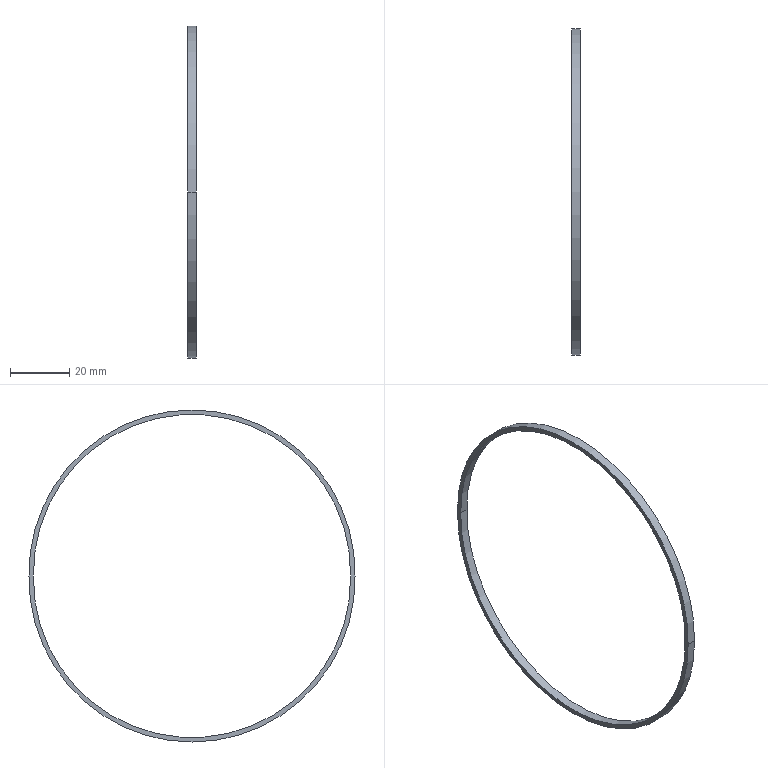Part | STEP file | 1-56.28 | 1 solid | 6 faces | box 3 x 110 x 112 mm | volume 1552 mm3 | cylinder 4 | plane 2 | commonest cylinder face diameters 107 x2 110 x2
STEP:
#1=CARTESIAN_POINT('',(0.,0.,0.));
#2=DIRECTION('',(0.,0.,1.));
#3=DIRECTION('',(1.,0.,0.));
#4=AXIS2_PLACEMENT_3D('',#1,#2,#3);
#5=CARTESIAN_POINT('',(0.,54.991,-1.));
#6=VERTEX_POINT('',#5);
#7=CARTESIAN_POINT('',(0.,-54.991,-1.));
#8=VERTEX_POINT('',#7);
#9=CARTESIAN_POINT('',(0.,0.,0.));
#10=DIRECTION('',(1.,0.,0.));
#11=DIRECTION('',(0.,0.9998,-0.01818));
#12=AXIS2_PLACEMENT_3D('',#9,#10,#11);
#13=CIRCLE('',#12,55.);
#14=CARTESIAN_POINT('',(0.,0.,-0.9907));
#15=DIRECTION('',(1.,0.,0.));
#16=DIRECTION('',(0.,1.,0.));
#17=AXIS2_PLACEMENT_3D('',#14,#15,#16);
#18=PLANE('',#17);
#19=CARTESIAN_POINT('',(0.,0.9907));
#20=DIRECTION('',(0.9998,-0.01818));
#21=AXIS2_PLACEMENT_2D('',#19,#20);
#22=CIRCLE('',#21,55.);
#23=(GEOMETRIC_REPRESENTATION_CONTEXT(2)PARAMETRIC_REPRESENTATION_CONTEXT()REPRESENTATION_CONTEXT('',''));
#24=DEFINITIONAL_REPRESENTATION('',(#22),#23);
#25=PCURVE('',#18,#24);
#26=CARTESIAN_POINT('',(0.,0.,0.));
#27=DIRECTION('',(1.,0.,0.));
#28=DIRECTION('',(0.,0.9998,-0.01818));
#29=AXIS2_PLACEMENT_3D('',#26,#27,#28);
#30=CYLINDRICAL_SURFACE('',#29,55.);
#31=CARTESIAN_POINT('',(0.,0.));
#32=DIRECTION('',(1.,0.));
#33=VECTOR('',#32,1.);
#34=LINE('',#31,#33);
#35=(GEOMETRIC_REPRESENTATION_CONTEXT(2)PARAMETRIC_REPRESENTATION_CONTEXT()REPRESENTATION_CONTEXT('',''));
#36=DEFINITIONAL_REPRESENTATION('',(#34),#35);
#37=PCURVE('',#30,#36);
#38=SURFACE_CURVE('',#13,(#25,#37),.PCURVE_S1.);
#39=EDGE_CURVE('',#6,#8,#38,.T.);
#40=ORIENTED_EDGE('',*,*,#39,.T.);
#41=CARTESIAN_POINT('',(0.,0.,-2.));
#42=DIRECTION('',(1.,0.,0.));
#43=DIRECTION('',(0.,-0.9998,0.01818));
#44=AXIS2_PLACEMENT_3D('',#41,#42,#43);
#45=CIRCLE('',#44,55.);
#46=CARTESIAN_POINT('',(0.,-1.009));
#47=DIRECTION('',(-0.9998,0.01818));
#48=AXIS2_PLACEMENT_2D('',#46,#47);
#49=CIRCLE('',#48,55.);
#50=(GEOMETRIC_REPRESENTATION_CONTEXT(2)PARAMETRIC_REPRESENTATION_CONTEXT()REPRESENTATION_CONTEXT('',''));
#51=DEFINITIONAL_REPRESENTATION('',(#49),#50);
#52=PCURVE('',#18,#51);
#53=CARTESIAN_POINT('',(0.,0.,-2.));
#54=DIRECTION('',(1.,0.,0.));
#55=DIRECTION('',(0.,-0.9998,0.01818));
#56=AXIS2_PLACEMENT_3D('',#53,#54,#55);
#57=CYLINDRICAL_SURFACE('',#56,55.);
#58=CARTESIAN_POINT('',(0.,0.));
#59=DIRECTION('',(1.,0.));
#60=VECTOR('',#59,1.);
#61=LINE('',#58,#60);
#62=(GEOMETRIC_REPRESENTATION_CONTEXT(2)PARAMETRIC_REPRESENTATION_CONTEXT()REPRESENTATION_CONTEXT('',''));
#63=DEFINITIONAL_REPRESENTATION('',(#61),#62);
#64=PCURVE('',#57,#63);
#65=SURFACE_CURVE('',#45,(#52,#64),.PCURVE_S1.);
#66=EDGE_CURVE('',#8,#6,#65,.T.);
#67=ORIENTED_EDGE('',*,*,#66,.T.);
#68=EDGE_LOOP('',(#40,#67));
#69=FACE_BOUND('',#68,.F.);
#70=CARTESIAN_POINT('',(0.,53.491,-1.));
#71=VERTEX_POINT('',#70);
#72=CARTESIAN_POINT('',(0.,-53.491,-1.));
#73=VERTEX_POINT('',#72);
#74=CARTESIAN_POINT('',(0.,0.,-2.));
#75=DIRECTION('',(-1.,0.,0.));
#76=DIRECTION('',(0.,0.9998,0.01869));
#77=AXIS2_PLACEMENT_3D('',#74,#75,#76);
#78=CIRCLE('',#77,53.5);
#79=CARTESIAN_POINT('',(53.491,-0.009258));
#80=CARTESIAN_POINT('',(55.223,-92.658));
#81=CARTESIAN_POINT('',(-25.879,-47.834));
#82=CARTESIAN_POINT('',(-106.981,-3.009));
#83=CARTESIAN_POINT('',(-27.611,44.815));
#84=CARTESIAN_POINT('',(51.759,92.639));
#85=CARTESIAN_POINT('',(53.491,-0.009258));
#86=(BOUNDED_CURVE()B_SPLINE_CURVE(2,(#79,#80,#81,#82,#83,#84,#85),.UNSPECIFIED.,.T.,.F.)B_SPLINE_CURVE_WITH_KNOTS((1,2,2,2,2,1),(-2.094,0.,2.094,4.189,6.283,8.378),.UNSPECIFIED.)CURVE()GEOMETRIC_REPRESENTATION_ITEM()RATIONAL_B_SPLINE_CURVE((1.,0.5,1.,0.5,1.,0.5,1.))REPRESENTATION_ITEM(''));
#87=(GEOMETRIC_REPRESENTATION_CONTEXT(2)PARAMETRIC_REPRESENTATION_CONTEXT()REPRESENTATION_CONTEXT('',''));
#88=DEFINITIONAL_REPRESENTATION('',(#86),#87);
#89=PCURVE('',#18,#88);
#90=CARTESIAN_POINT('',(0.,0.,-2.));
#91=DIRECTION('',(1.,0.,0.));
#92=DIRECTION('',(0.,0.9998,0.01869));
#93=AXIS2_PLACEMENT_3D('',#90,#91,#92);
#94=CYLINDRICAL_SURFACE('',#93,53.5);
#95=CARTESIAN_POINT('',(6.283,0.));
#96=DIRECTION('',(-1.,0.));
#97=VECTOR('',#96,1.);
#98=LINE('',#95,#97);
#99=(GEOMETRIC_REPRESENTATION_CONTEXT(2)PARAMETRIC_REPRESENTATION_CONTEXT()REPRESENTATION_CONTEXT('',''));
#100=DEFINITIONAL_REPRESENTATION('',(#98),#99);
#101=PCURVE('',#94,#100);
#102=SURFACE_CURVE('',#78,(#89,#101),.PCURVE_S1.);
#103=EDGE_CURVE('',#71,#73,#102,.T.);
#104=ORIENTED_EDGE('',*,*,#103,.T.);
#105=CARTESIAN_POINT('',(0.,0.,0.));
#106=DIRECTION('',(-1.,0.,0.));
#107=DIRECTION('',(0.,-0.9998,-0.01869));
#108=AXIS2_PLACEMENT_3D('',#105,#106,#107);
#109=CIRCLE('',#108,53.5);
#110=CARTESIAN_POINT('',(-53.491,-0.009258));
#111=CARTESIAN_POINT('',(-55.223,92.639));
#112=CARTESIAN_POINT('',(25.879,47.815));
#113=CARTESIAN_POINT('',(106.981,2.991));
#114=CARTESIAN_POINT('',(27.611,-44.834));
#115=CARTESIAN_POINT('',(-51.759,-92.658));
#116=CARTESIAN_POINT('',(-53.491,-0.009258));
#117=(BOUNDED_CURVE()B_SPLINE_CURVE(2,(#110,#111,#112,#113,#114,#115,#116),.UNSPECIFIED.,.T.,.F.)B_SPLINE_CURVE_WITH_KNOTS((1,2,2,2,2,1),(-2.094,0.,2.094,4.189,6.283,8.378),.UNSPECIFIED.)CURVE()GEOMETRIC_REPRESENTATION_ITEM()RATIONAL_B_SPLINE_CURVE((1.,0.5,1.,0.5,1.,0.5,1.))REPRESENTATION_ITEM(''));
#118=(GEOMETRIC_REPRESENTATION_CONTEXT(2)PARAMETRIC_REPRESENTATION_CONTEXT()REPRESENTATION_CONTEXT('',''));
#119=DEFINITIONAL_REPRESENTATION('',(#117),#118);
#120=PCURVE('',#18,#119);
#121=CARTESIAN_POINT('',(0.,0.,0.));
#122=DIRECTION('',(1.,0.,0.));
#123=DIRECTION('',(0.,-0.9998,-0.01869));
#124=AXIS2_PLACEMENT_3D('',#121,#122,#123);
#125=CYLINDRICAL_SURFACE('',#124,53.5);
#126=CARTESIAN_POINT('',(6.283,0.));
#127=DIRECTION('',(-1.,0.));
#128=VECTOR('',#127,1.);
#129=LINE('',#126,#128);
#130=(GEOMETRIC_REPRESENTATION_CONTEXT(2)PARAMETRIC_REPRESENTATION_CONTEXT()REPRESENTATION_CONTEXT('',''));
#131=DEFINITIONAL_REPRESENTATION('',(#129),#130);
#132=PCURVE('',#125,#131);
#133=SURFACE_CURVE('',#109,(#120,#132),.PCURVE_S1.);
#134=EDGE_CURVE('',#73,#71,#133,.T.);
#135=ORIENTED_EDGE('',*,*,#134,.T.);
#136=EDGE_LOOP('',(#104,#135));
#137=FACE_BOUND('',#136,.F.);
#138=ADVANCED_FACE('',(#69,#137),#18,.F.);
#139=CARTESIAN_POINT('',(3.,54.991,-1.));
#140=VERTEX_POINT('',#139);
#141=CARTESIAN_POINT('',(3.,-54.991,-1.));
#142=VERTEX_POINT('',#141);
#143=CARTESIAN_POINT('',(3.,0.,0.));
#144=DIRECTION('',(1.,0.,0.));
#145=DIRECTION('',(0.,0.9998,-0.01818));
#146=AXIS2_PLACEMENT_3D('',#143,#144,#145);
#147=CIRCLE('',#146,55.);
#148=CARTESIAN_POINT('',(3.,0.,-0.9907));
#149=DIRECTION('',(1.,0.,0.));
#150=DIRECTION('',(0.,1.,0.));
#151=AXIS2_PLACEMENT_3D('',#148,#149,#150);
#152=PLANE('',#151);
#153=CARTESIAN_POINT('',(0.,0.9907));
#154=DIRECTION('',(0.9998,-0.01818));
#155=AXIS2_PLACEMENT_2D('',#153,#154);
#156=CIRCLE('',#155,55.);
#157=(GEOMETRIC_REPRESENTATION_CONTEXT(2)PARAMETRIC_REPRESENTATION_CONTEXT()REPRESENTATION_CONTEXT('',''));
#158=DEFINITIONAL_REPRESENTATION('',(#156),#157);
#159=PCURVE('',#152,#158);
#160=CARTESIAN_POINT('',(0.,3.));
#161=DIRECTION('',(1.,0.));
#162=VECTOR('',#161,1.);
#163=LINE('',#160,#162);
#164=(GEOMETRIC_REPRESENTATION_CONTEXT(2)PARAMETRIC_REPRESENTATION_CONTEXT()REPRESENTATION_CONTEXT('',''));
#165=DEFINITIONAL_REPRESENTATION('',(#163),#164);
#166=PCURVE('',#30,#165);
#167=SURFACE_CURVE('',#147,(#159,#166),.PCURVE_S1.);
#168=EDGE_CURVE('',#140,#142,#167,.T.);
#169=ORIENTED_EDGE('',*,*,#168,.T.);
#170=CARTESIAN_POINT('',(3.,0.,-2.));
#171=DIRECTION('',(1.,0.,0.));
#172=DIRECTION('',(0.,-0.9998,0.01818));
#173=AXIS2_PLACEMENT_3D('',#170,#171,#172);
#174=CIRCLE('',#173,55.);
#175=CARTESIAN_POINT('',(0.,-1.009));
#176=DIRECTION('',(-0.9998,0.01818));
#177=AXIS2_PLACEMENT_2D('',#175,#176);
#178=CIRCLE('',#177,55.);
#179=(GEOMETRIC_REPRESENTATION_CONTEXT(2)PARAMETRIC_REPRESENTATION_CONTEXT()REPRESENTATION_CONTEXT('',''));
#180=DEFINITIONAL_REPRESENTATION('',(#178),#179);
#181=PCURVE('',#152,#180);
#182=CARTESIAN_POINT('',(0.,3.));
#183=DIRECTION('',(1.,0.));
#184=VECTOR('',#183,1.);
#185=LINE('',#182,#184);
#186=(GEOMETRIC_REPRESENTATION_CONTEXT(2)PARAMETRIC_REPRESENTATION_CONTEXT()REPRESENTATION_CONTEXT('',''));
#187=DEFINITIONAL_REPRESENTATION('',(#185),#186);
#188=PCURVE('',#57,#187);
#189=SURFACE_CURVE('',#174,(#181,#188),.PCURVE_S1.);
#190=EDGE_CURVE('',#142,#140,#189,.T.);
#191=ORIENTED_EDGE('',*,*,#190,.T.);
#192=EDGE_LOOP('',(#169,#191));
#193=FACE_BOUND('',#192,.T.);
#194=CARTESIAN_POINT('',(3.,53.491,-1.));
#195=VERTEX_POINT('',#194);
#196=CARTESIAN_POINT('',(3.,-53.491,-1.));
#197=VERTEX_POINT('',#196);
#198=CARTESIAN_POINT('',(3.,0.,-2.));
#199=DIRECTION('',(-1.,0.,0.));
#200=DIRECTION('',(0.,0.9998,0.01869));
#201=AXIS2_PLACEMENT_3D('',#198,#199,#200);
#202=CIRCLE('',#201,53.5);
#203=CARTESIAN_POINT('',(53.491,-0.009258));
#204=CARTESIAN_POINT('',(55.223,-92.658));
#205=CARTESIAN_POINT('',(-25.879,-47.834));
#206=CARTESIAN_POINT('',(-106.981,-3.009));
#207=CARTESIAN_POINT('',(-27.611,44.815));
#208=CARTESIAN_POINT('',(51.759,92.639));
#209=CARTESIAN_POINT('',(53.491,-0.009258));
#210=(BOUNDED_CURVE()B_SPLINE_CURVE(2,(#203,#204,#205,#206,#207,#208,#209),.UNSPECIFIED.,.T.,.F.)B_SPLINE_CURVE_WITH_KNOTS((1,2,2,2,2,1),(-2.094,0.,2.094,4.189,6.283,8.378),.UNSPECIFIED.)CURVE()GEOMETRIC_REPRESENTATION_ITEM()RATIONAL_B_SPLINE_CURVE((1.,0.5,1.,0.5,1.,0.5,1.))REPRESENTATION_ITEM(''));
#211=(GEOMETRIC_REPRESENTATION_CONTEXT(2)PARAMETRIC_REPRESENTATION_CONTEXT()REPRESENTATION_CONTEXT('',''));
#212=DEFINITIONAL_REPRESENTATION('',(#210),#211);
#213=PCURVE('',#152,#212);
#214=CARTESIAN_POINT('',(6.283,3.));
#215=DIRECTION('',(-1.,0.));
#216=VECTOR('',#215,1.);
#217=LINE('',#214,#216);
#218=(GEOMETRIC_REPRESENTATION_CONTEXT(2)PARAMETRIC_REPRESENTATION_CONTEXT()REPRESENTATION_CONTEXT('',''));
#219=DEFINITIONAL_REPRESENTATION('',(#217),#218);
#220=PCURVE('',#94,#219);
#221=SURFACE_CURVE('',#202,(#213,#220),.PCURVE_S1.);
#222=EDGE_CURVE('',#195,#197,#221,.T.);
#223=ORIENTED_EDGE('',*,*,#222,.T.);
#224=CARTESIAN_POINT('',(3.,0.,0.));
#225=DIRECTION('',(-1.,0.,0.));
#226=DIRECTION('',(0.,-0.9998,-0.01869));
#227=AXIS2_PLACEMENT_3D('',#224,#225,#226);
#228=CIRCLE('',#227,53.5);
#229=CARTESIAN_POINT('',(-53.491,-0.009258));
#230=CARTESIAN_POINT('',(-55.223,92.639));
#231=CARTESIAN_POINT('',(25.879,47.815));
#232=CARTESIAN_POINT('',(106.981,2.991));
#233=CARTESIAN_POINT('',(27.611,-44.834));
#234=CARTESIAN_POINT('',(-51.759,-92.658));
#235=CARTESIAN_POINT('',(-53.491,-0.009258));
#236=(BOUNDED_CURVE()B_SPLINE_CURVE(2,(#229,#230,#231,#232,#233,#234,#235),.UNSPECIFIED.,.T.,.F.)B_SPLINE_CURVE_WITH_KNOTS((1,2,2,2,2,1),(-2.094,0.,2.094,4.189,6.283,8.378),.UNSPECIFIED.)CURVE()GEOMETRIC_REPRESENTATION_ITEM()RATIONAL_B_SPLINE_CURVE((1.,0.5,1.,0.5,1.,0.5,1.))REPRESENTATION_ITEM(''));
#237=(GEOMETRIC_REPRESENTATION_CONTEXT(2)PARAMETRIC_REPRESENTATION_CONTEXT()REPRESENTATION_CONTEXT('',''));
#238=DEFINITIONAL_REPRESENTATION('',(#236),#237);
#239=PCURVE('',#152,#238);
#240=CARTESIAN_POINT('',(6.283,3.));
#241=DIRECTION('',(-1.,0.));
#242=VECTOR('',#241,1.);
#243=LINE('',#240,#242);
#244=(GEOMETRIC_REPRESENTATION_CONTEXT(2)PARAMETRIC_REPRESENTATION_CONTEXT()REPRESENTATION_CONTEXT('',''));
#245=DEFINITIONAL_REPRESENTATION('',(#243),#244);
#246=PCURVE('',#125,#245);
#247=SURFACE_CURVE('',#228,(#239,#246),.PCURVE_S1.);
#248=EDGE_CURVE('',#197,#195,#247,.T.);
#249=ORIENTED_EDGE('',*,*,#248,.T.);
#250=EDGE_LOOP('',(#223,#249));
#251=FACE_BOUND('',#250,.T.);
#252=ADVANCED_FACE('',(#193,#251),#152,.T.);
#253=ORIENTED_EDGE('',*,*,#39,.T.);
#254=CARTESIAN_POINT('',(0.,-54.991,-1.));
#255=DIRECTION('',(1.,0.,0.));
#256=VECTOR('',#255,1.);
#257=LINE('',#254,#256);
#258=CARTESIAN_POINT('',(3.178,0.));
#259=DIRECTION('',(0.,1.));
#260=VECTOR('',#259,1.);
#261=LINE('',#258,#260);
#262=(GEOMETRIC_REPRESENTATION_CONTEXT(2)PARAMETRIC_REPRESENTATION_CONTEXT()REPRESENTATION_CONTEXT('',''));
#263=DEFINITIONAL_REPRESENTATION('',(#261),#262);
#264=PCURVE('',#30,#263);
#265=CARTESIAN_POINT('',(0.,0.));
#266=DIRECTION('',(0.,1.));
#267=VECTOR('',#266,1.);
#268=LINE('',#265,#267);
#269=(GEOMETRIC_REPRESENTATION_CONTEXT(2)PARAMETRIC_REPRESENTATION_CONTEXT()REPRESENTATION_CONTEXT('',''));
#270=DEFINITIONAL_REPRESENTATION('',(#268),#269);
#271=PCURVE('',#57,#270);
#272=SURFACE_CURVE('',#257,(#264,#271),.PCURVE_S1.);
#273=EDGE_CURVE('',#8,#142,#272,.T.);
#274=ORIENTED_EDGE('',*,*,#273,.T.);
#275=ORIENTED_EDGE('',*,*,#168,.F.);
#276=CARTESIAN_POINT('',(0.,54.991,-1.));
#277=DIRECTION('',(1.,0.,0.));
#278=VECTOR('',#277,1.);
#279=LINE('',#276,#278);
#280=CARTESIAN_POINT('',(0.,0.));
#281=DIRECTION('',(0.,1.));
#282=VECTOR('',#281,1.);
#283=LINE('',#280,#282);
#284=(GEOMETRIC_REPRESENTATION_CONTEXT(2)PARAMETRIC_REPRESENTATION_CONTEXT()REPRESENTATION_CONTEXT('',''));
#285=DEFINITIONAL_REPRESENTATION('',(#283),#284);
#286=PCURVE('',#30,#285);
#287=CARTESIAN_POINT('',(3.178,0.));
#288=DIRECTION('',(0.,1.));
#289=VECTOR('',#288,1.);
#290=LINE('',#287,#289);
#291=(GEOMETRIC_REPRESENTATION_CONTEXT(2)PARAMETRIC_REPRESENTATION_CONTEXT()REPRESENTATION_CONTEXT('',''));
#292=DEFINITIONAL_REPRESENTATION('',(#290),#291);
#293=PCURVE('',#57,#292);
#294=SURFACE_CURVE('',#279,(#286,#293),.PCURVE_S1.);
#295=EDGE_CURVE('',#6,#140,#294,.T.);
#296=ORIENTED_EDGE('',*,*,#295,.F.);
#297=EDGE_LOOP('',(#253,#274,#275,#296));
#298=FACE_BOUND('',#297,.T.);
#299=ADVANCED_FACE('',(#298),#30,.T.);
#300=ORIENTED_EDGE('',*,*,#66,.T.);
#301=ORIENTED_EDGE('',*,*,#295,.T.);
#302=ORIENTED_EDGE('',*,*,#190,.F.);
#303=ORIENTED_EDGE('',*,*,#273,.F.);
#304=EDGE_LOOP('',(#300,#301,#302,#303));
#305=FACE_BOUND('',#304,.T.);
#306=ADVANCED_FACE('',(#305),#57,.T.);
#307=CARTESIAN_POINT('',(0.,53.491,-1.));
#308=DIRECTION('',(1.,0.,0.));
#309=VECTOR('',#308,1.);
#310=LINE('',#307,#309);
#311=CARTESIAN_POINT('',(6.283,0.));
#312=DIRECTION('',(0.,1.));
#313=VECTOR('',#312,1.);
#314=LINE('',#311,#313);
#315=(GEOMETRIC_REPRESENTATION_CONTEXT(2)PARAMETRIC_REPRESENTATION_CONTEXT()REPRESENTATION_CONTEXT('',''));
#316=DEFINITIONAL_REPRESENTATION('',(#314),#315);
#317=PCURVE('',#94,#316);
#318=CARTESIAN_POINT('',(3.104,0.));
#319=DIRECTION('',(0.,1.));
#320=VECTOR('',#319,1.);
#321=LINE('',#318,#320);
#322=(GEOMETRIC_REPRESENTATION_CONTEXT(2)PARAMETRIC_REPRESENTATION_CONTEXT()REPRESENTATION_CONTEXT('',''));
#323=DEFINITIONAL_REPRESENTATION('',(#321),#322);
#324=PCURVE('',#125,#323);
#325=SURFACE_CURVE('',#310,(#317,#324),.PCURVE_S1.);
#326=EDGE_CURVE('',#71,#195,#325,.T.);
#327=ORIENTED_EDGE('',*,*,#326,.T.);
#328=ORIENTED_EDGE('',*,*,#222,.T.);
#329=CARTESIAN_POINT('',(0.,-53.491,-1.));
#330=DIRECTION('',(1.,0.,0.));
#331=VECTOR('',#330,1.);
#332=LINE('',#329,#331);
#333=CARTESIAN_POINT('',(3.104,0.));
#334=DIRECTION('',(0.,1.));
#335=VECTOR('',#334,1.);
#336=LINE('',#333,#335);
#337=(GEOMETRIC_REPRESENTATION_CONTEXT(2)PARAMETRIC_REPRESENTATION_CONTEXT()REPRESENTATION_CONTEXT('',''));
#338=DEFINITIONAL_REPRESENTATION('',(#336),#337);
#339=PCURVE('',#94,#338);
#340=CARTESIAN_POINT('',(6.283,0.));
#341=DIRECTION('',(0.,1.));
#342=VECTOR('',#341,1.);
#343=LINE('',#340,#342);
#344=(GEOMETRIC_REPRESENTATION_CONTEXT(2)PARAMETRIC_REPRESENTATION_CONTEXT()REPRESENTATION_CONTEXT('',''));
#345=DEFINITIONAL_REPRESENTATION('',(#343),#344);
#346=PCURVE('',#125,#345);
#347=SURFACE_CURVE('',#332,(#339,#346),.PCURVE_S1.);
#348=EDGE_CURVE('',#73,#197,#347,.T.);
#349=ORIENTED_EDGE('',*,*,#348,.F.);
#350=ORIENTED_EDGE('',*,*,#103,.F.);
#351=EDGE_LOOP('',(#327,#328,#349,#350));
#352=FACE_BOUND('',#351,.F.);
#353=ADVANCED_FACE('',(#352),#94,.F.);
#354=ORIENTED_EDGE('',*,*,#348,.T.);
#355=ORIENTED_EDGE('',*,*,#248,.T.);
#356=ORIENTED_EDGE('',*,*,#326,.F.);
#357=ORIENTED_EDGE('',*,*,#134,.F.);
#358=EDGE_LOOP('',(#354,#355,#356,#357));
#359=FACE_BOUND('',#358,.F.);
#360=ADVANCED_FACE('',(#359),#125,.F.);
#361=CLOSED_SHELL('',(#138,#252,#299,#306,#353,#360));
#362=MANIFOLD_SOLID_BREP('',#361);
#363=(LENGTH_UNIT()NAMED_UNIT(*)SI_UNIT(.MILLI.,.METRE.));
#364=UNCERTAINTY_MEASURE_WITH_UNIT(LENGTH_MEASURE(0.0000001),#363,'','');
#365=(NAMED_UNIT(*)PLANE_ANGLE_UNIT()SI_UNIT($,.RADIAN.));
#366=(NAMED_UNIT(*)SI_UNIT($,.STERADIAN.)SOLID_ANGLE_UNIT());
#367=(GEOMETRIC_REPRESENTATION_CONTEXT(3)GLOBAL_UNCERTAINTY_ASSIGNED_CONTEXT((#364))GLOBAL_UNIT_ASSIGNED_CONTEXT((#363,#365,#366))REPRESENTATION_CONTEXT('',''));
#368=ADVANCED_BREP_SHAPE_REPRESENTATION('',(#4,#362),#367);